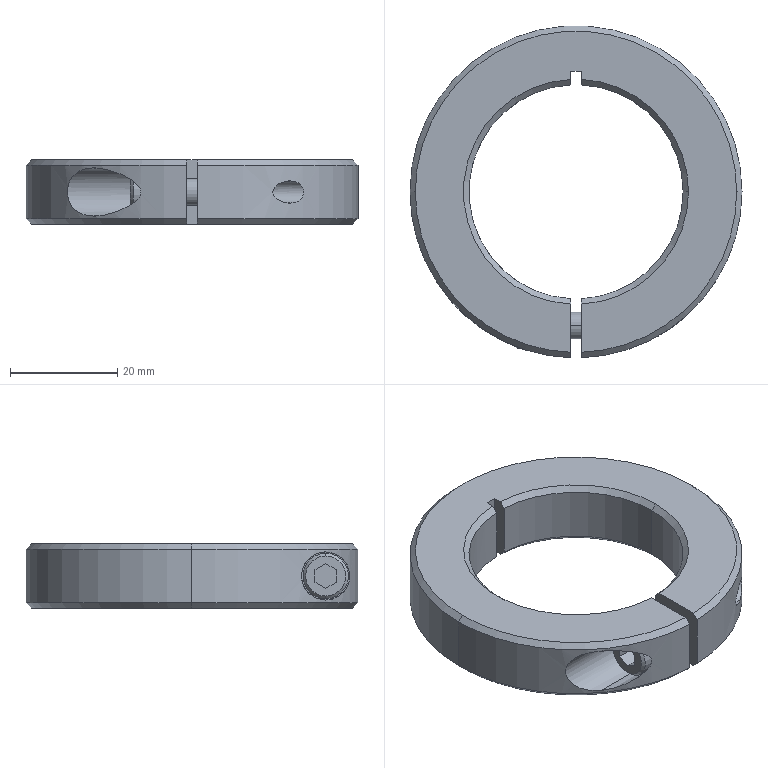Part | SolidWorks | features BaseBody 1 | 1 solid | 50 faces | box 62 x 61.984 x 12 mm | volume 19964 mm3 | plane 18 | cone 16 | cylinder 16 | commonest cylinder face diameters 40 x3 62 x3 4.134 x2 5 x2 5.5 x2 8.5 x2